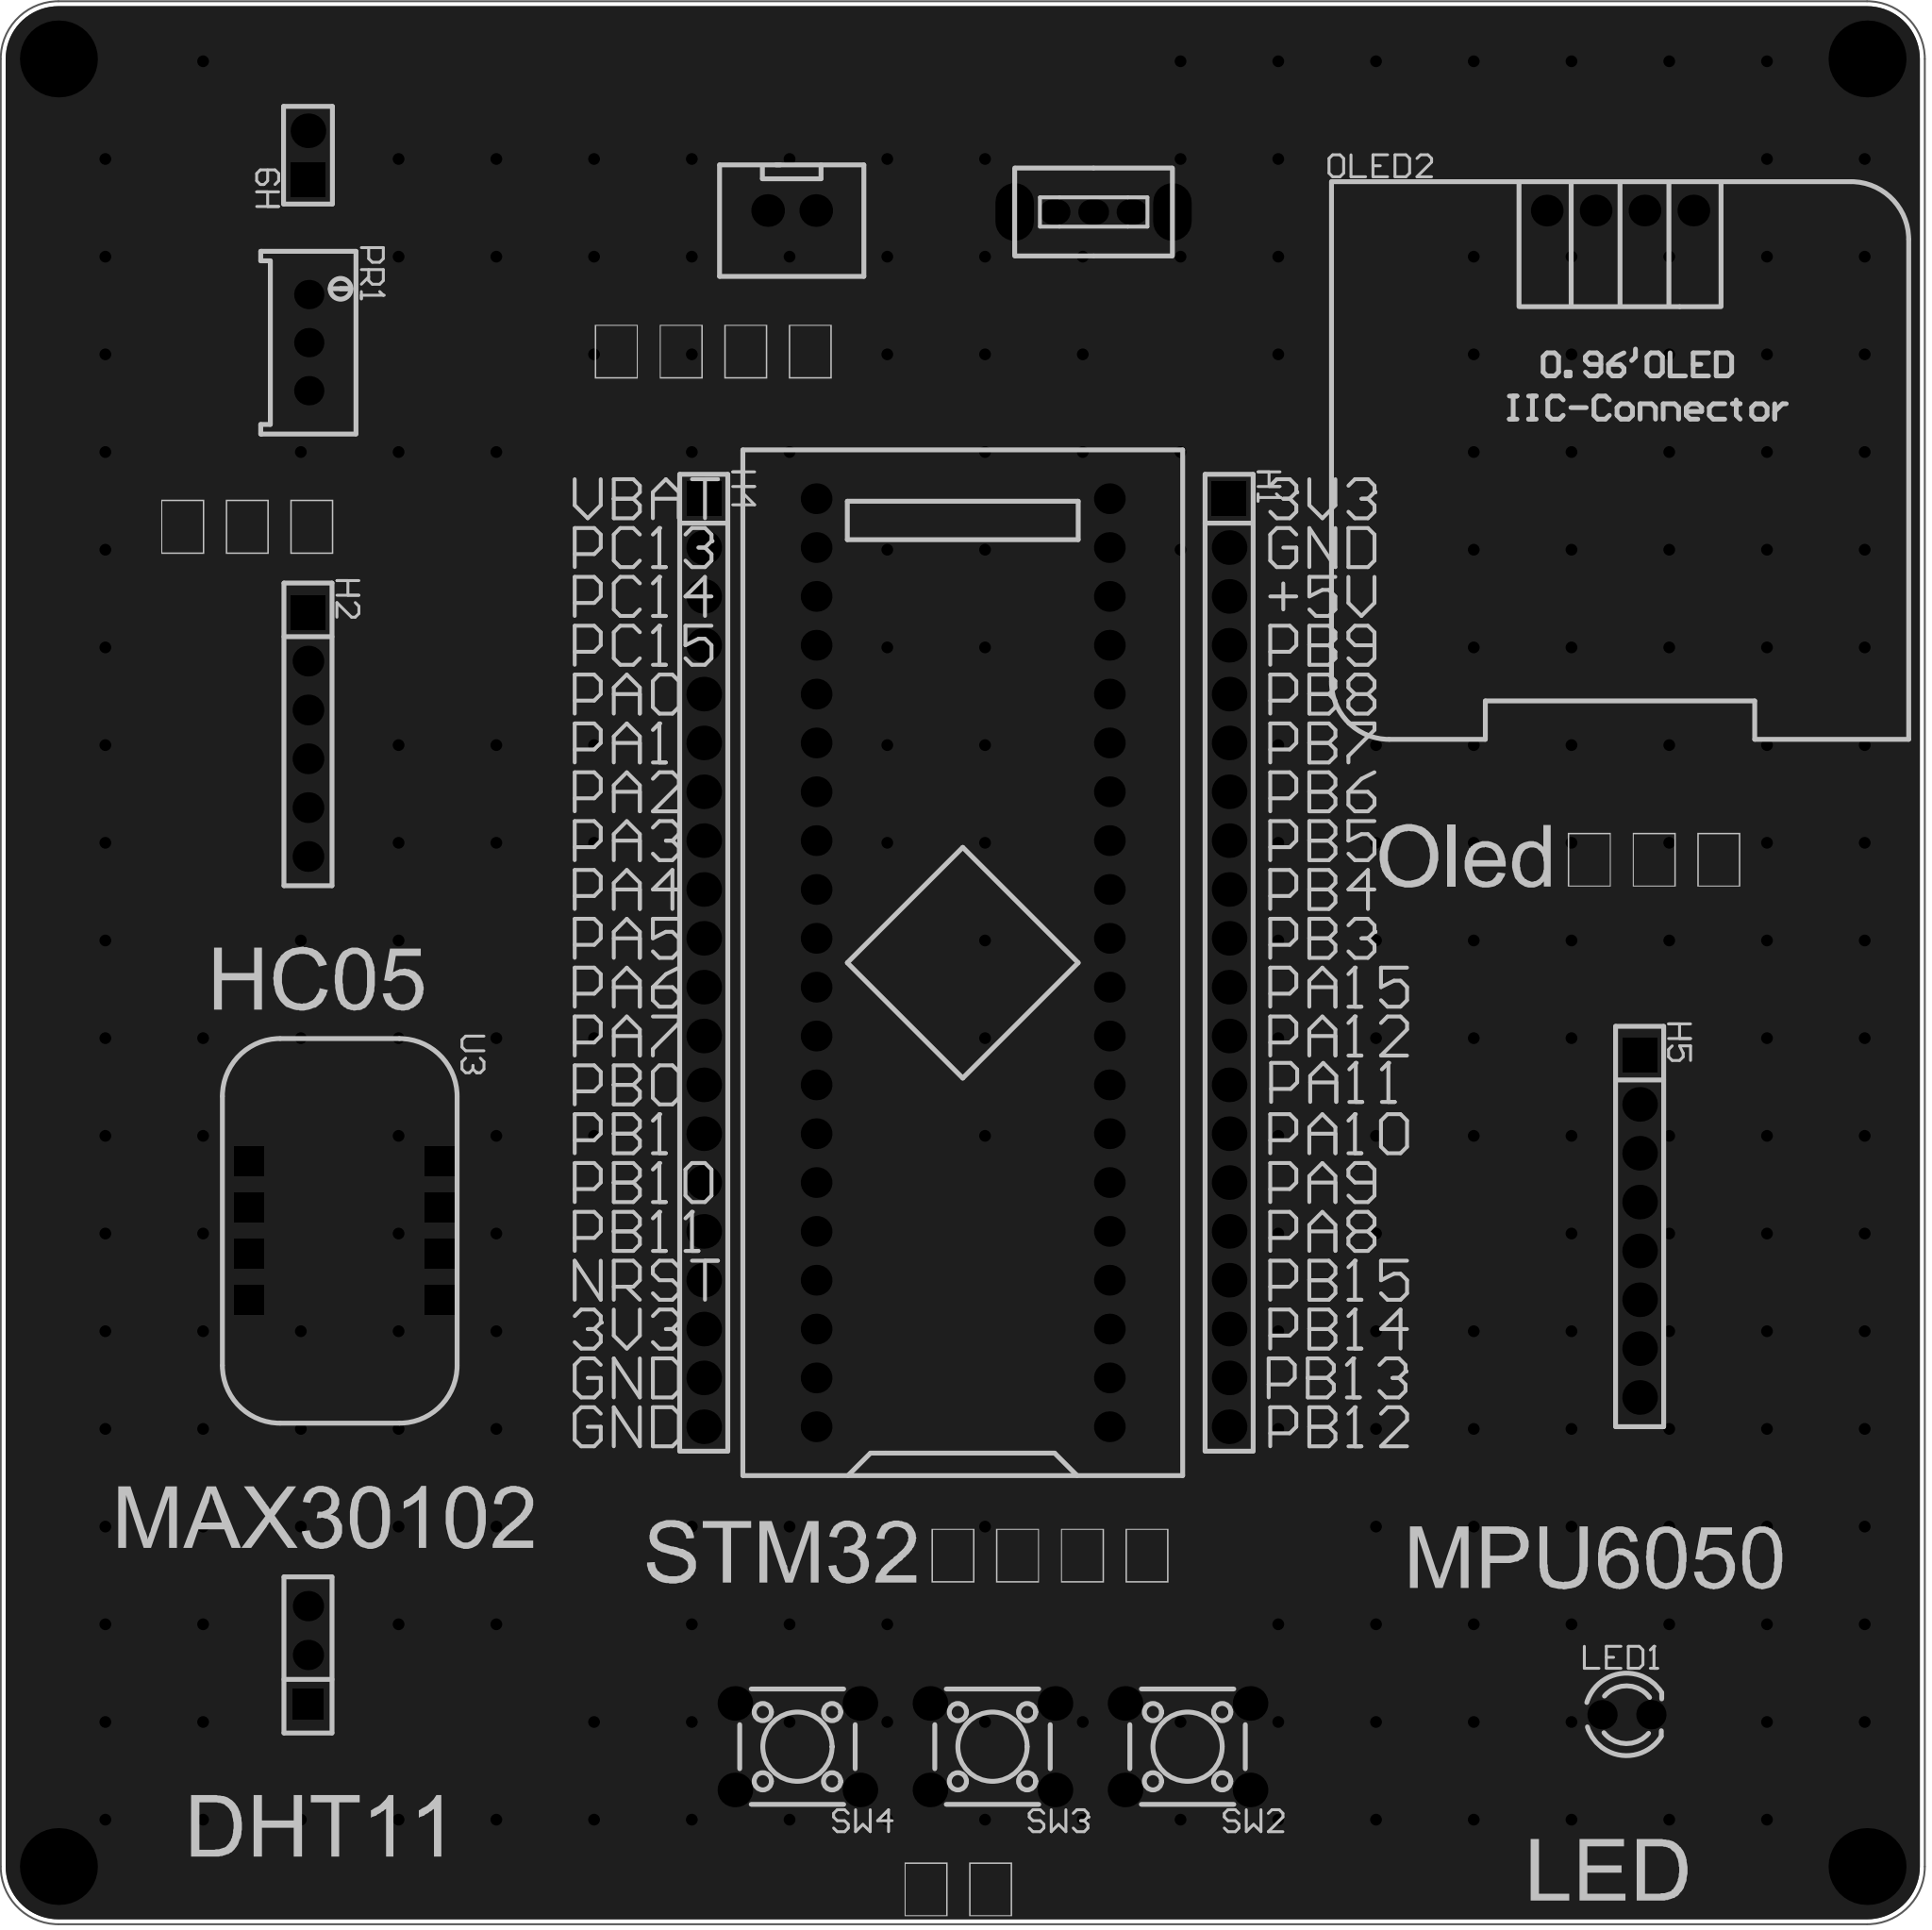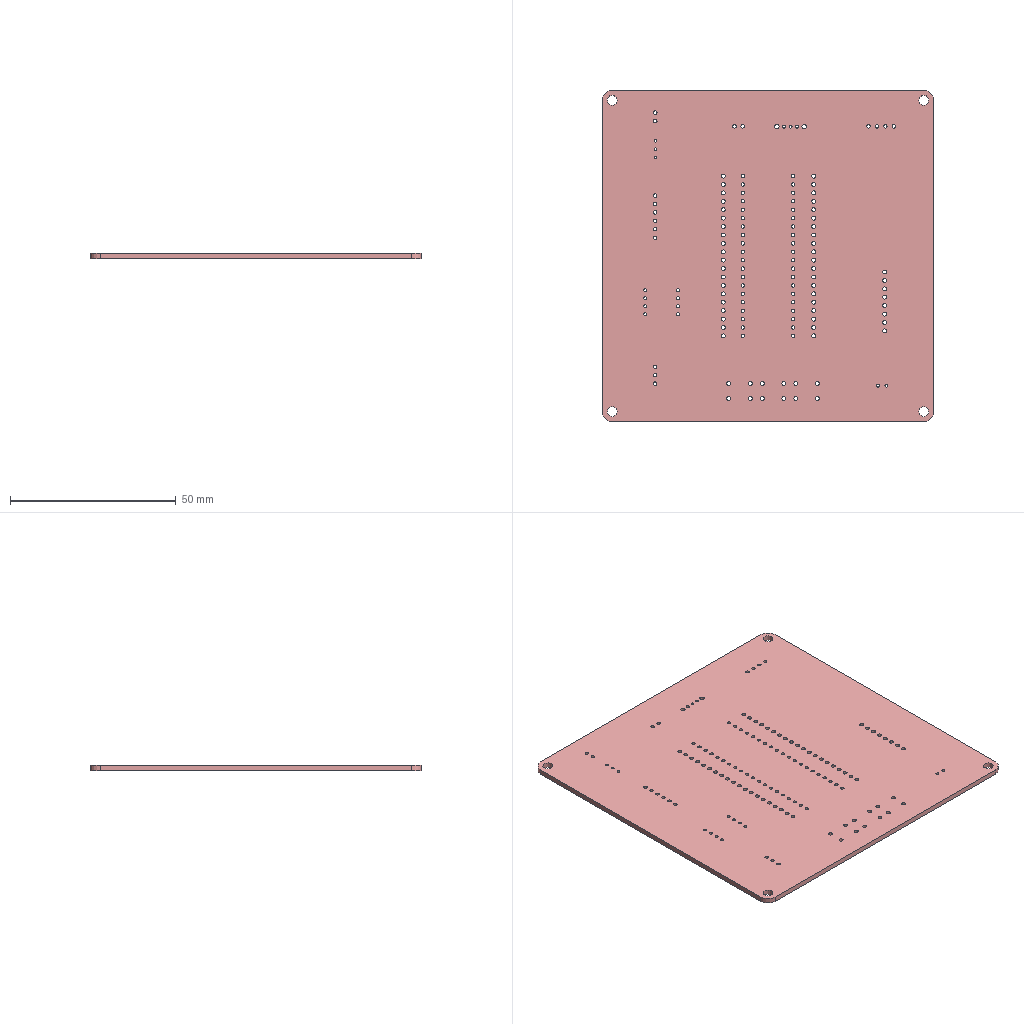Circuit board layout | Altium Designer | box 100 x 100 x 1.6 mm
Layer stack:
# Altium Designer layer stack of  (unit mm; dielectric type: 0 none, 1 core, 2 prepreg, 3 surface material)
index,name,kind,layer,copper_thickness_mm,dielectric_type,dielectric_thickness_mm,dielectric_material,dielectric_constant
0,Top Paste Mask Layer,other,,,,,,
1,Top Silkscreen Layer,other,,,,,,
2,Top Solder Mask Layer,dielectric,,,3,0.01,,3.3
3,Top Layer,copper,Top Layer,0.035,,,,
4,Dielectric1,dielectric,,,3,1.51,FR4,4.5
5,Bottom Layer,copper,Bottom Layer,0.035,,,,
6,Bottom Solder Mask Layer,dielectric,,,3,0.01,,3.3
7,Bottom Silkscreen Layer,other,,,,,,
8,Bottom Paste Mask Layer,other,,,,,,
# drill layer pairs: low layer,high layer
drill_pair,Top Layer,Bottom Layer
Part placement:
Designator,Comment,Layer,Footprint,Center-X(mm),Center-Y(mm),Rotation
U1,STM32F103C8T6-Card,TopLayer,CONN-TH_L53.3-W22.9_STM32F103C8T6-CARD,141.351,130.937,90
SW2,,TopLayer,SW-TH_4P-L6.0-W6.0-P4.50-LS6.5,153.035,90.17,180
SW3,,TopLayer,SW-TH_4P-L6.0-W6.0-P4.50-LS6.5,142.897,90.17,180
SW4,,TopLayer,SW-TH_4P-L6.0-W6.0-P4.50-LS6.5,132.759,90.17,180
CN4,XH2.54*2P_直插,TopLayer,CONN-TH_2P-P2.50-XH2.54-2P,132.461,170.053,0
SW5,,TopLayer,拨动开关,148.148,169.978,180
H3,,TopLayer,HDR-TH_3P-P2.54-V-F,107.32,94.94,90
H2,,TopLayer,HDR-TH_6P-P2.54-V-F,107.32,142.813,270
OLED2,,TopLayer,0.96OLED_4P,175.514,170.053,0
H9,,TopLayer,HDR-TH_2P-P2.54-V-M-1,107.32,172.931,90
LED1,,TopLayer,LED_TH-3mm,175.847,91.834,0
PR1,10kΩ,TopLayer,R_3296,107.363,163.185,270
U3,MAX30102,TopLayer,MAX30102,109.228,116.994,270
H1,,TopLayer,HDR-TH_20P-P2.54-V-M-1,155.194,130.937,270
H4,,TopLayer,HDR-TH_20P-P2.54-V-M-1,127.889,130.937,270
H5,,TopLayer,HDR-TH_8P-P2.54-V-F-1,176.53,117.221,270
Pad and via stacks:
# Altium Designer via and pad stacks of  (unit mm). Each distinct definition once, with the count of objects using it.
# via: kind,start_layer,end_layer,hole_mm,diameter_mm,mode(0 simple;1 top-mid-bottom;2 full stack),diameter_per_layer,count,example_net
# pad: kind,layer,hole_mm,hole_type(0 round;1 square;2 slot),plating,top_size,top_shape(1 round;2 rect;3 octagon;9 rounded rect),mid_size,bottom_size,mode,footprint,size_per_layer,count,example
pad,Multi-Layer,3,0,plated,4x4,1,4x4,4x4,0,,,4,1
pad,Multi-Layer,1,0,plated,1.6x1.6,1,1.6x1.6,1.6x1.6,0,CONN-TH_L53.3-W22.9_STM32F103C8T6-CARD,,40,U1.1
pad,Multi-Layer,1.2,0,plated,1.8x1.8,1,1.8x1.8,1.8x1.8,0,SW-TH_4P-L6.0-W6.0-P4.50-LS6.5,,12,SW2.1
pad,Multi-Layer,1.05,0,plated,1.7x1.7,1,1.7x1.7,1.7x1.7,0,CONN-TH_2P-P2.50-XH2.54-2P,,2,CN4.2
pad,Multi-Layer,0.8992,0,plated,1.6x1.3,1,1.6x1.3,1.6x1.3,0,\u00B2\u00A6\u00B6\u00AF\u00BF\u00AA\u00B9\u00D8,,3,SW5.1
pad,Multi-Layer,1.3,0,plated,3x1.999,1,3x1.999,3x1.999,0,\u00B2\u00A6\u00B6\u00AF\u00BF\u00AA\u00B9\u00D8,,2,SW5.4
pad,Multi-Layer,1.02,0,plated,1.575x1.575,1,1.575x1.575,1.575x1.575,0,HDR-TH_3P-P2.54-V-F,,2,H3.3
pad,Multi-Layer,1.02,0,plated,1.575x1.575,2,1.575x1.575,1.575x1.575,0,HDR-TH_3P-P2.54-V-F,,1,H3.1
pad,Multi-Layer,1.02,0,plated,1.6x1.6,1,1.6x1.6,1.6x1.6,0,HDR-TH_6P-P2.54-V-F,,5,H2.6
pad,Multi-Layer,1.02,0,plated,1.8x1.8,2,1.8x1.8,1.8x1.8,0,HDR-TH_6P-P2.54-V-F,,1,H2.1
pad,Multi-Layer,1,0,plated,1.65x1.65,1,1.65x1.65,1.65x1.65,0,0.96OLED_4P,,4,OLED2.4
pad,Multi-Layer,1.1,0,plated,1.8x1.8,1,1.8x1.8,1.8x1.8,0,HDR-TH_2P-P2.54-V-M-1,,1,H9.2
pad,Multi-Layer,1.1,0,plated,1.8x1.8,2,1.8x1.8,1.8x1.8,0,HDR-TH_2P-P2.54-V-M-1,,1,H9.1
pad,Multi-Layer,0.9144,0,plated,1.524x1.524,1,1.524x1.524,1.524x1.524,0,LED_TH-3mm,,2,LED1.1
pad,Multi-Layer,0.762,0,plated,1.524x1.524,1,1.524x1.524,1.524x1.524,0,R_3296,,3,PR1.2
pad,Multi-Layer,0.9144,0,plated,1.524x1.524,2,1.524x1.524,1.524x1.524,0,MAX30102,,8,U3.1
pad,Multi-Layer,1.2,0,plated,1.8x1.8,1,1.8x1.8,1.8x1.8,0,HDR-TH_20P-P2.54-V-M-1,,38,H1.20
pad,Multi-Layer,1.2,0,plated,1.8x1.8,2,1.8x1.8,1.8x1.8,0,HDR-TH_20P-P2.54-V-M-1,,2,H1.1
pad,Multi-Layer,1.2,0,plated,1.8x1.8,2,1.8x1.8,1.8x1.8,0,HDR-TH_8P-P2.54-V-F-1,,1,H5.1
pad,Multi-Layer,1.2,0,plated,1.8x1.8,1,1.8x1.8,1.8x1.8,0,HDR-TH_8P-P2.54-V-F-1,,7,H5.2
via,Top Layer,Bottom Layer,0.3048,0.61,0,,237,GND
Copper pours:
name,layer,net,type(0 solid;1 hatched;2 none)
Bottom Layer-GND,Bottom Layer,GND,0
Top Layer-GND,Top Layer,GND,0
Design rules, without the lines most boards share:
# Altium Designer design rules of  (exported by Altium Designer, unit mm)
# columns: name | kind | enabled | priority | scope1 | scope2 | descriptor | typed fields (field=value)
Copper_copperRegion_copperThickness1oz | 0 | disabled | 4 | All | All | Clearance Constraint (Gap=5.984mil) (Disabled)(All),(All) | gap=0.152
Copper_copperRegion_copperThickness1oz_1 | 63 | disabled | 4 | All | All | Board Clearance Constraint (Gap=0mil) (Disabled)(All) |
Copper_copperRegion_Copper_copperRegion | 0 | disabled | 5 | All | All | Clearance Constraint (Gap=5.984mil) (Disabled)(All),(All) | gap=0.152
Copper_copperRegion_Copper_copperRegion_1 | 63 | disabled | 5 | All | All | Board Clearance Constraint (Gap=0mil) (Disabled)(All) |
copperThickness1oz | 0 | enabled | 6 | All | All | Clearance Constraint (Gap=5.984mil) (All),(All) | gap=0.152
copperThickness1oz_1 | 63 | enabled | 6 | All | All | Board Clearance Constraint (Gap=0mil) (All) |
copperRegion_copperThickness1oz | 20 | disabled | 1 | All | All | Polygon Connect Rule(Relief Connect )(Conductor Width=10mil) (Relief Angle=90 Angle) (Entries=4) (Air Gap Width=10mil) (Disabled)(All),(All) | connect_style(0=relief,1=direct,2=none)=0 relief_conductor_width=0.254 relief_entries=4
copperRegion_Copper_copperRegion | 20 | disabled | 2 | All | All | Polygon Connect Rule(Relief Connect )(Conductor Width=10mil) (Relief Angle=90 Angle) (Entries=4) (Air Gap Width=10mil) (Disabled)(All),(All) | connect_style(0=relief,1=direct,2=none)=0 relief_conductor_width=0.254 relief_entries=4
copperRegion | 20 | enabled | 3 | All | All | Polygon Connect Rule(Relief Connect )(Conductor Width=10mil) (Relief Angle=90 Angle) (Entries=4) (Air Gap Width=10mil) (All),(All) | connect_style(0=relief,1=direct,2=none)=0 relief_conductor_width=0.254 relief_entries=4